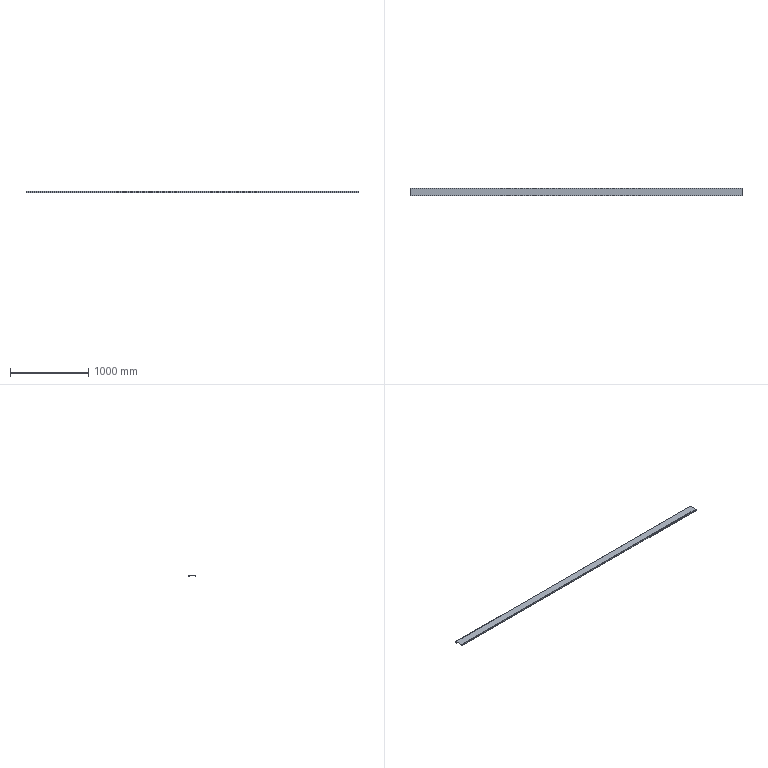Part | STEP file | E3-粉仓踢脚Plate 8 | 1 solid | 18 faces | box 4230 x 100 x 20 mm | volume 972350 mm3 | plane 12 | cylinder 6 | commonest cylinder face diameters 2 x3 5 x3
STEP:
#1=CARTESIAN_POINT('',(0.,0.,0.));
#2=DIRECTION('',(0.,0.,1.));
#3=DIRECTION('',(1.,0.,0.));
#4=AXIS2_PLACEMENT_3D('',#1,#2,#3);
#5=CARTESIAN_POINT('',(-2115.,1.5,-2.5));
#6=VERTEX_POINT('',#5);
#7=CARTESIAN_POINT('',(-2115.,1.5,-20.));
#8=VERTEX_POINT('',#7);
#9=CARTESIAN_POINT('',(-2115.,1.5,-2.5));
#10=DIRECTION('',(0.,0.,-1.));
#11=VECTOR('',#10,1.);
#12=LINE('',#9,#11);
#13=CARTESIAN_POINT('',(2115.,1.5,-2.5));
#14=DIRECTION('',(0.,-1.,0.));
#15=DIRECTION('',(0.,0.,1.));
#16=AXIS2_PLACEMENT_3D('',#13,#14,#15);
#17=PLANE('',#16);
#18=CARTESIAN_POINT('',(0.,4230.));
#19=DIRECTION('',(-1.,0.));
#20=VECTOR('',#19,1.);
#21=LINE('',#18,#20);
#22=(GEOMETRIC_REPRESENTATION_CONTEXT(2)PARAMETRIC_REPRESENTATION_CONTEXT()REPRESENTATION_CONTEXT('',''));
#23=DEFINITIONAL_REPRESENTATION('',(#21),#22);
#24=PCURVE('',#17,#23);
#25=CARTESIAN_POINT('',(-2115.,2.5,-2.5));
#26=DIRECTION('',(-1.,0.,0.));
#27=DIRECTION('',(0.,0.,-1.));
#28=AXIS2_PLACEMENT_3D('',#25,#26,#27);
#29=PLANE('',#28);
#30=CARTESIAN_POINT('',(0.,1.));
#31=DIRECTION('',(1.,0.));
#32=VECTOR('',#31,1.);
#33=LINE('',#30,#32);
#34=(GEOMETRIC_REPRESENTATION_CONTEXT(2)PARAMETRIC_REPRESENTATION_CONTEXT()REPRESENTATION_CONTEXT('',''));
#35=DEFINITIONAL_REPRESENTATION('',(#33),#34);
#36=PCURVE('',#29,#35);
#37=SURFACE_CURVE('',#12,(#24,#36),.PCURVE_S1.);
#38=EDGE_CURVE('',#6,#8,#37,.T.);
#39=ORIENTED_EDGE('',*,*,#38,.F.);
#40=CARTESIAN_POINT('',(2115.,1.5,-2.5));
#41=VERTEX_POINT('',#40);
#42=CARTESIAN_POINT('',(2115.,1.5,-2.5));
#43=DIRECTION('',(-1.,0.,0.));
#44=VECTOR('',#43,1.);
#45=LINE('',#42,#44);
#46=CARTESIAN_POINT('',(0.,0.));
#47=DIRECTION('',(0.,1.));
#48=VECTOR('',#47,1.);
#49=LINE('',#46,#48);
#50=(GEOMETRIC_REPRESENTATION_CONTEXT(2)PARAMETRIC_REPRESENTATION_CONTEXT()REPRESENTATION_CONTEXT('',''));
#51=DEFINITIONAL_REPRESENTATION('',(#49),#50);
#52=PCURVE('',#17,#51);
#53=CARTESIAN_POINT('',(2115.,2.5,-2.5));
#54=DIRECTION('',(-1.,0.,0.));
#55=DIRECTION('',(0.,0.,-1.));
#56=AXIS2_PLACEMENT_3D('',#53,#54,#55);
#57=CYLINDRICAL_SURFACE('',#56,1.);
#58=CARTESIAN_POINT('',(1.571,0.));
#59=DIRECTION('',(0.,1.));
#60=VECTOR('',#59,1.);
#61=LINE('',#58,#60);
#62=(GEOMETRIC_REPRESENTATION_CONTEXT(2)PARAMETRIC_REPRESENTATION_CONTEXT()REPRESENTATION_CONTEXT('',''));
#63=DEFINITIONAL_REPRESENTATION('',(#61),#62);
#64=PCURVE('',#57,#63);
#65=SURFACE_CURVE('',#45,(#52,#64),.PCURVE_S1.);
#66=EDGE_CURVE('',#41,#6,#65,.T.);
#67=ORIENTED_EDGE('',*,*,#66,.F.);
#68=CARTESIAN_POINT('',(2115.,1.5,-20.));
#69=VERTEX_POINT('',#68);
#70=CARTESIAN_POINT('',(2115.,1.5,-2.5));
#71=DIRECTION('',(0.,0.,-1.));
#72=VECTOR('',#71,1.);
#73=LINE('',#70,#72);
#74=CARTESIAN_POINT('',(0.,0.));
#75=DIRECTION('',(-1.,0.));
#76=VECTOR('',#75,1.);
#77=LINE('',#74,#76);
#78=(GEOMETRIC_REPRESENTATION_CONTEXT(2)PARAMETRIC_REPRESENTATION_CONTEXT()REPRESENTATION_CONTEXT('',''));
#79=DEFINITIONAL_REPRESENTATION('',(#77),#78);
#80=PCURVE('',#17,#79);
#81=CARTESIAN_POINT('',(2115.,2.5,-2.5));
#82=DIRECTION('',(-1.,0.,0.));
#83=DIRECTION('',(0.,0.,-1.));
#84=AXIS2_PLACEMENT_3D('',#81,#82,#83);
#85=PLANE('',#84);
#86=CARTESIAN_POINT('',(0.,1.));
#87=DIRECTION('',(1.,0.));
#88=VECTOR('',#87,1.);
#89=LINE('',#86,#88);
#90=(GEOMETRIC_REPRESENTATION_CONTEXT(2)PARAMETRIC_REPRESENTATION_CONTEXT()REPRESENTATION_CONTEXT('',''));
#91=DEFINITIONAL_REPRESENTATION('',(#89),#90);
#92=PCURVE('',#85,#91);
#93=SURFACE_CURVE('',#73,(#80,#92),.PCURVE_S1.);
#94=EDGE_CURVE('',#41,#69,#93,.T.);
#95=ORIENTED_EDGE('',*,*,#94,.T.);
#96=CARTESIAN_POINT('',(2115.,1.5,-20.));
#97=DIRECTION('',(-1.,0.,0.));
#98=VECTOR('',#97,1.);
#99=LINE('',#96,#98);
#100=CARTESIAN_POINT('',(-17.5,0.));
#101=DIRECTION('',(0.,1.));
#102=VECTOR('',#101,1.);
#103=LINE('',#100,#102);
#104=(GEOMETRIC_REPRESENTATION_CONTEXT(2)PARAMETRIC_REPRESENTATION_CONTEXT()REPRESENTATION_CONTEXT('',''));
#105=DEFINITIONAL_REPRESENTATION('',(#103),#104);
#106=PCURVE('',#17,#105);
#107=CARTESIAN_POINT('',(2115.,0.,-20.));
#108=DIRECTION('',(0.,0.,-1.));
#109=DIRECTION('',(1.,0.,0.));
#110=AXIS2_PLACEMENT_3D('',#107,#108,#109);
#111=PLANE('',#110);
#112=CARTESIAN_POINT('',(0.,-1.5));
#113=DIRECTION('',(-1.,0.));
#114=VECTOR('',#113,1.);
#115=LINE('',#112,#114);
#116=(GEOMETRIC_REPRESENTATION_CONTEXT(2)PARAMETRIC_REPRESENTATION_CONTEXT()REPRESENTATION_CONTEXT('',''));
#117=DEFINITIONAL_REPRESENTATION('',(#115),#116);
#118=PCURVE('',#111,#117);
#119=SURFACE_CURVE('',#99,(#106,#118),.PCURVE_S1.);
#120=EDGE_CURVE('',#69,#8,#119,.T.);
#121=ORIENTED_EDGE('',*,*,#120,.T.);
#122=EDGE_LOOP('',(#39,#67,#95,#121));
#123=FACE_BOUND('',#122,.T.);
#124=ADVANCED_FACE('',(#123),#17,.F.);
#125=CARTESIAN_POINT('',(-2115.,0.,-20.));
#126=VERTEX_POINT('',#125);
#127=CARTESIAN_POINT('',(-2115.,0.,-20.));
#128=DIRECTION('',(0.,1.,0.));
#129=VECTOR('',#128,1.);
#130=LINE('',#127,#129);
#131=CARTESIAN_POINT('',(-4230.,0.));
#132=DIRECTION('',(0.,-1.));
#133=VECTOR('',#132,1.);
#134=LINE('',#131,#133);
#135=(GEOMETRIC_REPRESENTATION_CONTEXT(2)PARAMETRIC_REPRESENTATION_CONTEXT()REPRESENTATION_CONTEXT('',''));
#136=DEFINITIONAL_REPRESENTATION('',(#134),#135);
#137=PCURVE('',#111,#136);
#138=CARTESIAN_POINT('',(17.5,2.5));
#139=DIRECTION('',(0.,-1.));
#140=VECTOR('',#139,1.);
#141=LINE('',#138,#140);
#142=(GEOMETRIC_REPRESENTATION_CONTEXT(2)PARAMETRIC_REPRESENTATION_CONTEXT()REPRESENTATION_CONTEXT('',''));
#143=DEFINITIONAL_REPRESENTATION('',(#141),#142);
#144=PCURVE('',#29,#143);
#145=SURFACE_CURVE('',#130,(#137,#144),.PCURVE_S1.);
#146=EDGE_CURVE('',#126,#8,#145,.T.);
#147=ORIENTED_EDGE('',*,*,#146,.T.);
#148=ORIENTED_EDGE('',*,*,#120,.F.);
#149=CARTESIAN_POINT('',(2115.,0.,-20.));
#150=VERTEX_POINT('',#149);
#151=CARTESIAN_POINT('',(2115.,0.,-20.));
#152=DIRECTION('',(0.,1.,0.));
#153=VECTOR('',#152,1.);
#154=LINE('',#151,#153);
#155=CARTESIAN_POINT('',(0.,0.));
#156=DIRECTION('',(0.,-1.));
#157=VECTOR('',#156,1.);
#158=LINE('',#155,#157);
#159=(GEOMETRIC_REPRESENTATION_CONTEXT(2)PARAMETRIC_REPRESENTATION_CONTEXT()REPRESENTATION_CONTEXT('',''));
#160=DEFINITIONAL_REPRESENTATION('',(#158),#159);
#161=PCURVE('',#111,#160);
#162=CARTESIAN_POINT('',(17.5,2.5));
#163=DIRECTION('',(0.,-1.));
#164=VECTOR('',#163,1.);
#165=LINE('',#162,#164);
#166=(GEOMETRIC_REPRESENTATION_CONTEXT(2)PARAMETRIC_REPRESENTATION_CONTEXT()REPRESENTATION_CONTEXT('',''));
#167=DEFINITIONAL_REPRESENTATION('',(#165),#166);
#168=PCURVE('',#85,#167);
#169=SURFACE_CURVE('',#154,(#161,#168),.PCURVE_S1.);
#170=EDGE_CURVE('',#150,#69,#169,.T.);
#171=ORIENTED_EDGE('',*,*,#170,.F.);
#172=CARTESIAN_POINT('',(2115.,0.,-20.));
#173=DIRECTION('',(-1.,0.,0.));
#174=VECTOR('',#173,1.);
#175=LINE('',#172,#174);
#176=CARTESIAN_POINT('',(0.,0.));
#177=DIRECTION('',(-1.,0.));
#178=VECTOR('',#177,1.);
#179=LINE('',#176,#178);
#180=(GEOMETRIC_REPRESENTATION_CONTEXT(2)PARAMETRIC_REPRESENTATION_CONTEXT()REPRESENTATION_CONTEXT('',''));
#181=DEFINITIONAL_REPRESENTATION('',(#179),#180);
#182=PCURVE('',#111,#181);
#183=CARTESIAN_POINT('',(2115.,0.,-2.5));
#184=DIRECTION('',(0.,-1.,0.));
#185=DIRECTION('',(0.,0.,1.));
#186=AXIS2_PLACEMENT_3D('',#183,#184,#185);
#187=PLANE('',#186);
#188=CARTESIAN_POINT('',(-17.5,0.));
#189=DIRECTION('',(0.,1.));
#190=VECTOR('',#189,1.);
#191=LINE('',#188,#190);
#192=(GEOMETRIC_REPRESENTATION_CONTEXT(2)PARAMETRIC_REPRESENTATION_CONTEXT()REPRESENTATION_CONTEXT('',''));
#193=DEFINITIONAL_REPRESENTATION('',(#191),#192);
#194=PCURVE('',#187,#193);
#195=SURFACE_CURVE('',#175,(#182,#194),.PCURVE_S1.);
#196=EDGE_CURVE('',#150,#126,#195,.T.);
#197=ORIENTED_EDGE('',*,*,#196,.T.);
#198=EDGE_LOOP('',(#147,#148,#171,#197));
#199=FACE_BOUND('',#198,.T.);
#200=ADVANCED_FACE('',(#199),#111,.T.);
#201=CARTESIAN_POINT('',(-2115.,0.,-2.5));
#202=VERTEX_POINT('',#201);
#203=CARTESIAN_POINT('',(-2115.,0.,-2.5));
#204=DIRECTION('',(0.,0.,-1.));
#205=VECTOR('',#204,1.);
#206=LINE('',#203,#205);
#207=CARTESIAN_POINT('',(0.,4230.));
#208=DIRECTION('',(-1.,0.));
#209=VECTOR('',#208,1.);
#210=LINE('',#207,#209);
#211=(GEOMETRIC_REPRESENTATION_CONTEXT(2)PARAMETRIC_REPRESENTATION_CONTEXT()REPRESENTATION_CONTEXT('',''));
#212=DEFINITIONAL_REPRESENTATION('',(#210),#211);
#213=PCURVE('',#187,#212);
#214=CARTESIAN_POINT('',(0.,2.5));
#215=DIRECTION('',(1.,0.));
#216=VECTOR('',#215,1.);
#217=LINE('',#214,#216);
#218=(GEOMETRIC_REPRESENTATION_CONTEXT(2)PARAMETRIC_REPRESENTATION_CONTEXT()REPRESENTATION_CONTEXT('',''));
#219=DEFINITIONAL_REPRESENTATION('',(#217),#218);
#220=PCURVE('',#29,#219);
#221=SURFACE_CURVE('',#206,(#213,#220),.PCURVE_S1.);
#222=EDGE_CURVE('',#202,#126,#221,.T.);
#223=ORIENTED_EDGE('',*,*,#222,.T.);
#224=ORIENTED_EDGE('',*,*,#196,.F.);
#225=CARTESIAN_POINT('',(2115.,0.,-2.5));
#226=VERTEX_POINT('',#225);
#227=CARTESIAN_POINT('',(2115.,0.,-2.5));
#228=DIRECTION('',(0.,0.,-1.));
#229=VECTOR('',#228,1.);
#230=LINE('',#227,#229);
#231=CARTESIAN_POINT('',(0.,0.));
#232=DIRECTION('',(-1.,0.));
#233=VECTOR('',#232,1.);
#234=LINE('',#231,#233);
#235=(GEOMETRIC_REPRESENTATION_CONTEXT(2)PARAMETRIC_REPRESENTATION_CONTEXT()REPRESENTATION_CONTEXT('',''));
#236=DEFINITIONAL_REPRESENTATION('',(#234),#235);
#237=PCURVE('',#187,#236);
#238=CARTESIAN_POINT('',(0.,2.5));
#239=DIRECTION('',(1.,0.));
#240=VECTOR('',#239,1.);
#241=LINE('',#238,#240);
#242=(GEOMETRIC_REPRESENTATION_CONTEXT(2)PARAMETRIC_REPRESENTATION_CONTEXT()REPRESENTATION_CONTEXT('',''));
#243=DEFINITIONAL_REPRESENTATION('',(#241),#242);
#244=PCURVE('',#85,#243);
#245=SURFACE_CURVE('',#230,(#237,#244),.PCURVE_S1.);
#246=EDGE_CURVE('',#226,#150,#245,.T.);
#247=ORIENTED_EDGE('',*,*,#246,.F.);
#248=CARTESIAN_POINT('',(2115.,0.,-2.5));
#249=DIRECTION('',(-1.,0.,0.));
#250=VECTOR('',#249,1.);
#251=LINE('',#248,#250);
#252=CARTESIAN_POINT('',(0.,0.));
#253=DIRECTION('',(0.,1.));
#254=VECTOR('',#253,1.);
#255=LINE('',#252,#254);
#256=(GEOMETRIC_REPRESENTATION_CONTEXT(2)PARAMETRIC_REPRESENTATION_CONTEXT()REPRESENTATION_CONTEXT('',''));
#257=DEFINITIONAL_REPRESENTATION('',(#255),#256);
#258=PCURVE('',#187,#257);
#259=CARTESIAN_POINT('',(2115.,2.5,-2.5));
#260=DIRECTION('',(-1.,0.,0.));
#261=DIRECTION('',(0.,0.,-1.));
#262=AXIS2_PLACEMENT_3D('',#259,#260,#261);
#263=CYLINDRICAL_SURFACE('',#262,2.5);
#264=CARTESIAN_POINT('',(1.571,0.));
#265=DIRECTION('',(0.,1.));
#266=VECTOR('',#265,1.);
#267=LINE('',#264,#266);
#268=(GEOMETRIC_REPRESENTATION_CONTEXT(2)PARAMETRIC_REPRESENTATION_CONTEXT()REPRESENTATION_CONTEXT('',''));
#269=DEFINITIONAL_REPRESENTATION('',(#267),#268);
#270=PCURVE('',#263,#269);
#271=SURFACE_CURVE('',#251,(#258,#270),.PCURVE_S1.);
#272=EDGE_CURVE('',#226,#202,#271,.T.);
#273=ORIENTED_EDGE('',*,*,#272,.T.);
#274=EDGE_LOOP('',(#223,#224,#247,#273));
#275=FACE_BOUND('',#274,.T.);
#276=ADVANCED_FACE('',(#275),#187,.T.);
#277=CARTESIAN_POINT('',(-2115.,2.5,0.));
#278=VERTEX_POINT('',#277);
#279=CARTESIAN_POINT('',(-2115.,2.5,-2.5));
#280=DIRECTION('',(1.,0.,0.));
#281=DIRECTION('',(0.,0.,-1.));
#282=AXIS2_PLACEMENT_3D('',#279,#280,#281);
#283=CIRCLE('',#282,2.5);
#284=CARTESIAN_POINT('',(6.283,4230.));
#285=DIRECTION('',(-1.,0.));
#286=VECTOR('',#285,1.);
#287=LINE('',#284,#286);
#288=(GEOMETRIC_REPRESENTATION_CONTEXT(2)PARAMETRIC_REPRESENTATION_CONTEXT()REPRESENTATION_CONTEXT('',''));
#289=DEFINITIONAL_REPRESENTATION('',(#287),#288);
#290=PCURVE('',#263,#289);
#291=CARTESIAN_POINT('',(2.5,0.));
#292=CARTESIAN_POINT('',(2.5,-4.33));
#293=CARTESIAN_POINT('',(-1.25,-2.165));
#294=CARTESIAN_POINT('',(-5.,0.));
#295=CARTESIAN_POINT('',(-1.25,2.165));
#296=CARTESIAN_POINT('',(2.5,4.33));
#297=CARTESIAN_POINT('',(2.5,0.));
#298=(BOUNDED_CURVE()B_SPLINE_CURVE(2,(#291,#292,#293,#294,#295,#296,#297),.UNSPECIFIED.,.T.,.F.)B_SPLINE_CURVE_WITH_KNOTS((1,2,2,2,2,1),(-2.094,0.,2.094,4.189,6.283,8.378),.UNSPECIFIED.)CURVE()GEOMETRIC_REPRESENTATION_ITEM()RATIONAL_B_SPLINE_CURVE((1.,0.5,1.,0.5,1.,0.5,1.))REPRESENTATION_ITEM(''));
#299=(GEOMETRIC_REPRESENTATION_CONTEXT(2)PARAMETRIC_REPRESENTATION_CONTEXT()REPRESENTATION_CONTEXT('',''));
#300=DEFINITIONAL_REPRESENTATION('',(#298),#299);
#301=PCURVE('',#29,#300);
#302=SURFACE_CURVE('',#283,(#290,#301),.PCURVE_S1.);
#303=EDGE_CURVE('',#278,#202,#302,.T.);
#304=ORIENTED_EDGE('',*,*,#303,.T.);
#305=ORIENTED_EDGE('',*,*,#272,.F.);
#306=CARTESIAN_POINT('',(2115.,2.5,0.));
#307=VERTEX_POINT('',#306);
#308=CARTESIAN_POINT('',(2115.,2.5,-2.5));
#309=DIRECTION('',(1.,0.,0.));
#310=DIRECTION('',(0.,0.,-1.));
#311=AXIS2_PLACEMENT_3D('',#308,#309,#310);
#312=CIRCLE('',#311,2.5);
#313=CARTESIAN_POINT('',(6.283,0.));
#314=DIRECTION('',(-1.,0.));
#315=VECTOR('',#314,1.);
#316=LINE('',#313,#315);
#317=(GEOMETRIC_REPRESENTATION_CONTEXT(2)PARAMETRIC_REPRESENTATION_CONTEXT()REPRESENTATION_CONTEXT('',''));
#318=DEFINITIONAL_REPRESENTATION('',(#316),#317);
#319=PCURVE('',#263,#318);
#320=CARTESIAN_POINT('',(2.5,0.));
#321=CARTESIAN_POINT('',(2.5,-4.33));
#322=CARTESIAN_POINT('',(-1.25,-2.165));
#323=CARTESIAN_POINT('',(-5.,0.));
#324=CARTESIAN_POINT('',(-1.25,2.165));
#325=CARTESIAN_POINT('',(2.5,4.33));
#326=CARTESIAN_POINT('',(2.5,0.));
#327=(BOUNDED_CURVE()B_SPLINE_CURVE(2,(#320,#321,#322,#323,#324,#325,#326),.UNSPECIFIED.,.T.,.F.)B_SPLINE_CURVE_WITH_KNOTS((1,2,2,2,2,1),(-2.094,0.,2.094,4.189,6.283,8.378),.UNSPECIFIED.)CURVE()GEOMETRIC_REPRESENTATION_ITEM()RATIONAL_B_SPLINE_CURVE((1.,0.5,1.,0.5,1.,0.5,1.))REPRESENTATION_ITEM(''));
#328=(GEOMETRIC_REPRESENTATION_CONTEXT(2)PARAMETRIC_REPRESENTATION_CONTEXT()REPRESENTATION_CONTEXT('',''));
#329=DEFINITIONAL_REPRESENTATION('',(#327),#328);
#330=PCURVE('',#85,#329);
#331=SURFACE_CURVE('',#312,(#319,#330),.PCURVE_S1.);
#332=EDGE_CURVE('',#307,#226,#331,.T.);
#333=ORIENTED_EDGE('',*,*,#332,.F.);
#334=CARTESIAN_POINT('',(2115.,2.5,0.));
#335=DIRECTION('',(-1.,0.,0.));
#336=VECTOR('',#335,1.);
#337=LINE('',#334,#336);
#338=CARTESIAN_POINT('',(3.142,0.));
#339=DIRECTION('',(0.,1.));
#340=VECTOR('',#339,1.);
#341=LINE('',#338,#340);
#342=(GEOMETRIC_REPRESENTATION_CONTEXT(2)PARAMETRIC_REPRESENTATION_CONTEXT()REPRESENTATION_CONTEXT('',''));
#343=DEFINITIONAL_REPRESENTATION('',(#341),#342);
#344=PCURVE('',#263,#343);
#345=CARTESIAN_POINT('',(2115.,2.5,0.));
#346=DIRECTION('',(0.,0.,1.));
#347=DIRECTION('',(-1.,0.,0.));
#348=AXIS2_PLACEMENT_3D('',#345,#346,#347);
#349=PLANE('',#348);
#350=CARTESIAN_POINT('',(0.,0.));
#351=DIRECTION('',(1.,0.));
#352=VECTOR('',#351,1.);
#353=LINE('',#350,#352);
#354=(GEOMETRIC_REPRESENTATION_CONTEXT(2)PARAMETRIC_REPRESENTATION_CONTEXT()REPRESENTATION_CONTEXT('',''));
#355=DEFINITIONAL_REPRESENTATION('',(#353),#354);
#356=PCURVE('',#349,#355);
#357=SURFACE_CURVE('',#337,(#344,#356),.PCURVE_S1.);
#358=EDGE_CURVE('',#307,#278,#357,.T.);
#359=ORIENTED_EDGE('',*,*,#358,.T.);
#360=EDGE_LOOP('',(#304,#305,#333,#359));
#361=FACE_BOUND('',#360,.T.);
#362=ADVANCED_FACE('',(#361),#263,.T.);
#363=CARTESIAN_POINT('',(-2115.,97.5,0.));
#364=VERTEX_POINT('',#363);
#365=CARTESIAN_POINT('',(-2115.,2.5,0.));
#366=DIRECTION('',(0.,-1.,0.));
#367=VECTOR('',#366,1.);
#368=LINE('',#365,#367);
#369=CARTESIAN_POINT('',(4230.,0.));
#370=DIRECTION('',(0.,1.));
#371=VECTOR('',#370,1.);
#372=LINE('',#369,#371);
#373=(GEOMETRIC_REPRESENTATION_CONTEXT(2)PARAMETRIC_REPRESENTATION_CONTEXT()REPRESENTATION_CONTEXT('',''));
#374=DEFINITIONAL_REPRESENTATION('',(#372),#373);
#375=PCURVE('',#349,#374);
#376=CARTESIAN_POINT('',(-2.5,0.));
#377=DIRECTION('',(0.,1.));
#378=VECTOR('',#377,1.);
#379=LINE('',#376,#378);
#380=(GEOMETRIC_REPRESENTATION_CONTEXT(2)PARAMETRIC_REPRESENTATION_CONTEXT()REPRESENTATION_CONTEXT('',''));
#381=DEFINITIONAL_REPRESENTATION('',(#379),#380);
#382=PCURVE('',#29,#381);
#383=SURFACE_CURVE('',#368,(#375,#382),.PCURVE_S1.);
#384=EDGE_CURVE('',#364,#278,#383,.T.);
#385=ORIENTED_EDGE('',*,*,#384,.T.);
#386=ORIENTED_EDGE('',*,*,#358,.F.);
#387=CARTESIAN_POINT('',(2115.,97.5,0.));
#388=VERTEX_POINT('',#387);
#389=CARTESIAN_POINT('',(2115.,2.5,0.));
#390=DIRECTION('',(0.,-1.,0.));
#391=VECTOR('',#390,1.);
#392=LINE('',#389,#391);
#393=CARTESIAN_POINT('',(0.,0.));
#394=DIRECTION('',(0.,1.));
#395=VECTOR('',#394,1.);
#396=LINE('',#393,#395);
#397=(GEOMETRIC_REPRESENTATION_CONTEXT(2)PARAMETRIC_REPRESENTATION_CONTEXT()REPRESENTATION_CONTEXT('',''));
#398=DEFINITIONAL_REPRESENTATION('',(#396),#397);
#399=PCURVE('',#349,#398);
#400=CARTESIAN_POINT('',(-2.5,0.));
#401=DIRECTION('',(0.,1.));
#402=VECTOR('',#401,1.);
#403=LINE('',#400,#402);
#404=(GEOMETRIC_REPRESENTATION_CONTEXT(2)PARAMETRIC_REPRESENTATION_CONTEXT()REPRESENTATION_CONTEXT('',''));
#405=DEFINITIONAL_REPRESENTATION('',(#403),#404);
#406=PCURVE('',#85,#405);
#407=SURFACE_CURVE('',#392,(#399,#406),.PCURVE_S1.);
#408=EDGE_CURVE('',#388,#307,#407,.T.);
#409=ORIENTED_EDGE('',*,*,#408,.F.);
#410=CARTESIAN_POINT('',(2115.,97.5,0.));
#411=DIRECTION('',(-1.,0.,0.));
#412=VECTOR('',#411,1.);
#413=LINE('',#410,#412);
#414=CARTESIAN_POINT('',(0.,-95.));
#415=DIRECTION('',(1.,0.));
#416=VECTOR('',#415,1.);
#417=LINE('',#414,#416);
#418=(GEOMETRIC_REPRESENTATION_CONTEXT(2)PARAMETRIC_REPRESENTATION_CONTEXT()REPRESENTATION_CONTEXT('',''));
#419=DEFINITIONAL_REPRESENTATION('',(#417),#418);
#420=PCURVE('',#349,#419);
#421=CARTESIAN_POINT('',(2115.,97.5,-2.5));
#422=DIRECTION('',(-1.,0.,0.));
#423=DIRECTION('',(0.,0.,-1.));
#424=AXIS2_PLACEMENT_3D('',#421,#422,#423);
#425=CYLINDRICAL_SURFACE('',#424,2.5);
#426=CARTESIAN_POINT('',(3.142,0.));
#427=DIRECTION('',(0.,1.));
#428=VECTOR('',#427,1.);
#429=LINE('',#426,#428);
#430=(GEOMETRIC_REPRESENTATION_CONTEXT(2)PARAMETRIC_REPRESENTATION_CONTEXT()REPRESENTATION_CONTEXT('',''));
#431=DEFINITIONAL_REPRESENTATION('',(#429),#430);
#432=PCURVE('',#425,#431);
#433=SURFACE_CURVE('',#413,(#420,#432),.PCURVE_S1.);
#434=EDGE_CURVE('',#388,#364,#433,.T.);
#435=ORIENTED_EDGE('',*,*,#434,.T.);
#436=EDGE_LOOP('',(#385,#386,#409,#435));
#437=FACE_BOUND('',#436,.T.);
#438=ADVANCED_FACE('',(#437),#349,.T.);
#439=CARTESIAN_POINT('',(-2115.,100.,-2.5));
#440=VERTEX_POINT('',#439);
#441=CARTESIAN_POINT('',(-2115.,97.5,-2.5));
#442=DIRECTION('',(1.,0.,0.));
#443=DIRECTION('',(0.,0.,1.));
#444=AXIS2_PLACEMENT_3D('',#441,#442,#443);
#445=CIRCLE('',#444,2.5);
#446=CARTESIAN_POINT('',(9.425,4230.));
#447=DIRECTION('',(-1.,0.));
#448=VECTOR('',#447,1.);
#449=LINE('',#446,#448);
#450=(GEOMETRIC_REPRESENTATION_CONTEXT(2)PARAMETRIC_REPRESENTATION_CONTEXT()REPRESENTATION_CONTEXT('',''));
#451=DEFINITIONAL_REPRESENTATION('',(#449),#450);
#452=PCURVE('',#425,#451);
#453=CARTESIAN_POINT('',(-2.5,-95.));
#454=CARTESIAN_POINT('',(-2.5,-90.67));
#455=CARTESIAN_POINT('',(1.25,-92.835));
#456=CARTESIAN_POINT('',(5.,-95.));
#457=CARTESIAN_POINT('',(1.25,-97.165));
#458=CARTESIAN_POINT('',(-2.5,-99.33));
#459=CARTESIAN_POINT('',(-2.5,-95.));
#460=(BOUNDED_CURVE()B_SPLINE_CURVE(2,(#453,#454,#455,#456,#457,#458,#459),.UNSPECIFIED.,.T.,.F.)B_SPLINE_CURVE_WITH_KNOTS((1,2,2,2,2,1),(-2.094,0.,2.094,4.189,6.283,8.378),.UNSPECIFIED.)CURVE()GEOMETRIC_REPRESENTATION_ITEM()RATIONAL_B_SPLINE_CURVE((1.,0.5,1.,0.5,1.,0.5,1.))REPRESENTATION_ITEM(''));
#461=(GEOMETRIC_REPRESENTATION_CONTEXT(2)PARAMETRIC_REPRESENTATION_CONTEXT()REPRESENTATION_CONTEXT('',''));
#462=DEFINITIONAL_REPRESENTATION('',(#460),#461);
#463=PCURVE('',#29,#462);
#464=SURFACE_CURVE('',#445,(#452,#463),.PCURVE_S1.);
#465=EDGE_CURVE('',#440,#364,#464,.T.);
#466=ORIENTED_EDGE('',*,*,#465,.T.);
#467=ORIENTED_EDGE('',*,*,#434,.F.);
#468=CARTESIAN_POINT('',(2115.,100.,-2.5));
#469=VERTEX_POINT('',#468);
#470=CARTESIAN_POINT('',(2115.,97.5,-2.5));
#471=DIRECTION('',(1.,0.,0.));
#472=DIRECTION('',(0.,0.,1.));
#473=AXIS2_PLACEMENT_3D('',#470,#471,#472);
#474=CIRCLE('',#473,2.5);
#475=CARTESIAN_POINT('',(9.425,0.));
#476=DIRECTION('',(-1.,0.));
#477=VECTOR('',#476,1.);
#478=LINE('',#475,#477);
#479=(GEOMETRIC_REPRESENTATION_CONTEXT(2)PARAMETRIC_REPRESENTATION_CONTEXT()REPRESENTATION_CONTEXT('',''));
#480=DEFINITIONAL_REPRESENTATION('',(#478),#479);
#481=PCURVE('',#425,#480);
#482=CARTESIAN_POINT('',(-2.5,-95.));
#483=CARTESIAN_POINT('',(-2.5,-90.67));
#484=CARTESIAN_POINT('',(1.25,-92.835));
#485=CARTESIAN_POINT('',(5.,-95.));
#486=CARTESIAN_POINT('',(1.25,-97.165));
#487=CARTESIAN_POINT('',(-2.5,-99.33));
#488=CARTESIAN_POINT('',(-2.5,-95.));
#489=(BOUNDED_CURVE()B_SPLINE_CURVE(2,(#482,#483,#484,#485,#486,#487,#488),.UNSPECIFIED.,.T.,.F.)B_SPLINE_CURVE_WITH_KNOTS((1,2,2,2,2,1),(-2.094,0.,2.094,4.189,6.283,8.378),.UNSPECIFIED.)CURVE()GEOMETRIC_REPRESENTATION_ITEM()RATIONAL_B_SPLINE_CURVE((1.,0.5,1.,0.5,1.,0.5,1.))REPRESENTATION_ITEM(''));
#490=(GEOMETRIC_REPRESENTATION_CONTEXT(2)PARAMETRIC_REPRESENTATION_CONTEXT()REPRESENTATION_CONTEXT('',''));
#491=DEFINITIONAL_REPRESENTATION('',(#489),#490);
#492=PCURVE('',#85,#491);
#493=SURFACE_CURVE('',#474,(#481,#492),.PCURVE_S1.);
#494=EDGE_CURVE('',#469,#388,#493,.T.);
#495=ORIENTED_EDGE('',*,*,#494,.F.);
#496=CARTESIAN_POINT('',(2115.,100.,-2.5));
#497=DIRECTION('',(-1.,0.,0.));
#498=VECTOR('',#497,1.);
#499=LINE('',#496,#498);
#500=CARTESIAN_POINT('',(4.712,0.));
#501=DIRECTION('',(0.,1.));
#502=VECTOR('',#501,1.);
#503=LINE('',#500,#502);
#504=(GEOMETRIC_REPRESENTATION_CONTEXT(2)PARAMETRIC_REPRESENTATION_CONTEXT()REPRESENTATION_CONTEXT('',''));
#505=DEFINITIONAL_REPRESENTATION('',(#503),#504);
#506=PCURVE('',#425,#505);
#507=CARTESIAN_POINT('',(2115.,100.,-2.5));
#508=DIRECTION('',(0.,1.,0.));
#509=DIRECTION('',(0.,0.,-1.));
#510=AXIS2_PLACEMENT_3D('',#507,#508,#509);
#511=PLANE('',#510);
#512=CARTESIAN_POINT('',(0.,0.));
#513=DIRECTION('',(0.,1.));
#514=VECTOR('',#513,1.);
#515=LINE('',#512,#514);
#516=(GEOMETRIC_REPRESENTATION_CONTEXT(2)PARAMETRIC_REPRESENTATION_CONTEXT()REPRESENTATION_CONTEXT('',''));
#517=DEFINITIONAL_REPRESENTATION('',(#515),#516);
#518=PCURVE('',#511,#517);
#519=SURFACE_CURVE('',#499,(#506,#518),.PCURVE_S1.);
#520=EDGE_CURVE('',#469,#440,#519,.T.);
#521=ORIENTED_EDGE('',*,*,#520,.T.);
#522=EDGE_LOOP('',(#466,#467,#495,#521));
#523=FACE_BOUND('',#522,.T.);
#524=ADVANCED_FACE('',(#523),#425,.T.);
#525=CARTESIAN_POINT('',(-2115.,100.,-17.5));
#526=VERTEX_POINT('',#525);
#527=CARTESIAN_POINT('',(-2115.,100.,-2.5));
#528=DIRECTION('',(0.,0.,1.));
#529=VECTOR('',#528,1.);
#530=LINE('',#527,#529);
#531=CARTESIAN_POINT('',(0.,4230.));
#532=DIRECTION('',(-1.,0.));
#533=VECTOR('',#532,1.);
#534=LINE('',#531,#533);
#535=(GEOMETRIC_REPRESENTATION_CONTEXT(2)PARAMETRIC_REPRESENTATION_CONTEXT()REPRESENTATION_CONTEXT('',''));
#536=DEFINITIONAL_REPRESENTATION('',(#534),#535);
#537=PCURVE('',#511,#536);
#538=CARTESIAN_POINT('',(0.,-97.5));
#539=DIRECTION('',(-1.,0.));
#540=VECTOR('',#539,1.);
#541=LINE('',#538,#540);
#542=(GEOMETRIC_REPRESENTATION_CONTEXT(2)PARAMETRIC_REPRESENTATION_CONTEXT()REPRESENTATION_CONTEXT('',''));
#543=DEFINITIONAL_REPRESENTATION('',(#541),#542);
#544=PCURVE('',#29,#543);
#545=SURFACE_CURVE('',#530,(#537,#544),.PCURVE_S1.);
#546=EDGE_CURVE('',#526,#440,#545,.T.);
#547=ORIENTED_EDGE('',*,*,#546,.T.);
#548=ORIENTED_EDGE('',*,*,#520,.F.);
#549=CARTESIAN_POINT('',(2115.,100.,-17.5));
#550=VERTEX_POINT('',#549);
#551=CARTESIAN_POINT('',(2115.,100.,-2.5));
#552=DIRECTION('',(0.,0.,1.));
#553=VECTOR('',#552,1.);
#554=LINE('',#551,#553);
#555=CARTESIAN_POINT('',(0.,0.));
#556=DIRECTION('',(-1.,0.));
#557=VECTOR('',#556,1.);
#558=LINE('',#555,#557);
#559=(GEOMETRIC_REPRESENTATION_CONTEXT(2)PARAMETRIC_REPRESENTATION_CONTEXT()REPRESENTATION_CONTEXT('',''));
#560=DEFINITIONAL_REPRESENTATION('',(#558),#559);
#561=PCURVE('',#511,#560);
#562=CARTESIAN_POINT('',(0.,-97.5));
#563=DIRECTION('',(-1.,0.));
#564=VECTOR('',#563,1.);
#565=LINE('',#562,#564);
#566=(GEOMETRIC_REPRESENTATION_CONTEXT(2)PARAMETRIC_REPRESENTATION_CONTEXT()REPRESENTATION_CONTEXT('',''));
#567=DEFINITIONAL_REPRESENTATION('',(#565),#566);
#568=PCURVE('',#85,#567);
#569=SURFACE_CURVE('',#554,(#561,#568),.PCURVE_S1.);
#570=EDGE_CURVE('',#550,#469,#569,.T.);
#571=ORIENTED_EDGE('',*,*,#570,.F.);
#572=CARTESIAN_POINT('',(2115.,100.,-17.5));
#573=DIRECTION('',(-1.,0.,0.));
#574=VECTOR('',#573,1.);
#575=LINE('',#572,#574);
#576=CARTESIAN_POINT('',(15.,0.));
#577=DIRECTION('',(0.,1.));
#578=VECTOR('',#577,1.);
#579=LINE('',#576,#578);
#580=(GEOMETRIC_REPRESENTATION_CONTEXT(2)PARAMETRIC_REPRESENTATION_CONTEXT()REPRESENTATION_CONTEXT('',''));
#581=DEFINITIONAL_REPRESENTATION('',(#579),#580);
#582=PCURVE('',#511,#581);
#583=CARTESIAN_POINT('',(2115.,97.5,-17.5));
#584=DIRECTION('',(-1.,0.,0.));
#585=DIRECTION('',(0.,0.,-1.));
#586=AXIS2_PLACEMENT_3D('',#583,#584,#585);
#587=CYLINDRICAL_SURFACE('',#586,2.5);
#588=CARTESIAN_POINT('',(4.712,0.));
#589=DIRECTION('',(0.,1.));
#590=VECTOR('',#589,1.);
#591=LINE('',#588,#590);
#592=(GEOMETRIC_REPRESENTATION_CONTEXT(2)PARAMETRIC_REPRESENTATION_CONTEXT()REPRESENTATION_CONTEXT('',''));
#593=DEFINITIONAL_REPRESENTATION('',(#591),#592);
#594=PCURVE('',#587,#593);
#595=SURFACE_CURVE('',#575,(#582,#594),.PCURVE_S1.);
#596=EDGE_CURVE('',#550,#526,#595,.T.);
#597=ORIENTED_EDGE('',*,*,#596,.T.);
#598=EDGE_LOOP('',(#547,#548,#571,#597));
#599=FACE_BOUND('',#598,.T.);
#600=ADVANCED_FACE('',(#599),#511,.T.);
#601=CARTESIAN_POINT('',(-2115.,97.5,-20.));
#602=VERTEX_POINT('',#601);
#603=CARTESIAN_POINT('',(-2115.,97.5,-17.5));
#604=DIRECTION('',(1.,0.,0.));
#605=DIRECTION('',(0.,0.,1.));
#606=AXIS2_PLACEMENT_3D('',#603,#604,#605);
#607=CIRCLE('',#606,2.5);
#608=CARTESIAN_POINT('',(9.425,4230.));
#609=DIRECTION('',(-1.,0.));
#610=VECTOR('',#609,1.);
#611=LINE('',#608,#610);
#612=(GEOMETRIC_REPRESENTATION_CONTEXT(2)PARAMETRIC_REPRESENTATION_CONTEXT()REPRESENTATION_CONTEXT('',''));
#613=DEFINITIONAL_REPRESENTATION('',(#611),#612);
#614=PCURVE('',#587,#613);
#615=CARTESIAN_POINT('',(12.5,-95.));
#616=CARTESIAN_POINT('',(12.5,-90.67));
#617=CARTESIAN_POINT('',(16.25,-92.835));
#618=CARTESIAN_POINT('',(20.,-95.));
#619=CARTESIAN_POINT('',(16.25,-97.165));
#620=CARTESIAN_POINT('',(12.5,-99.33));
#621=CARTESIAN_POINT('',(12.5,-95.));
#622=(BOUNDED_CURVE()B_SPLINE_CURVE(2,(#615,#616,#617,#618,#619,#620,#621),.UNSPECIFIED.,.T.,.F.)B_SPLINE_CURVE_WITH_KNOTS((1,2,2,2,2,1),(-2.094,0.,2.094,4.189,6.283,8.378),.UNSPECIFIED.)CURVE()GEOMETRIC_REPRESENTATION_ITEM()RATIONAL_B_SPLINE_CURVE((1.,0.5,1.,0.5,1.,0.5,1.))REPRESENTATION_ITEM(''));
#623=(GEOMETRIC_REPRESENTATION_CONTEXT(2)PARAMETRIC_REPRESENTATION_CONTEXT()REPRESENTATION_CONTEXT('',''));
#624=DEFINITIONAL_REPRESENTATION('',(#622),#623);
#625=PCURVE('',#29,#624);
#626=SURFACE_CURVE('',#607,(#614,#625),.PCURVE_S1.);
#627=EDGE_CURVE('',#602,#526,#626,.T.);
#628=ORIENTED_EDGE('',*,*,#627,.T.);
#629=ORIENTED_EDGE('',*,*,#596,.F.);
#630=CARTESIAN_POINT('',(2115.,97.5,-20.));
#631=VERTEX_POINT('',#630);
#632=CARTESIAN_POINT('',(2115.,97.5,-17.5));
#633=DIRECTION('',(1.,0.,0.));
#634=DIRECTION('',(0.,0.,1.));
#635=AXIS2_PLACEMENT_3D('',#632,#633,#634);
#636=CIRCLE('',#635,2.5);
#637=CARTESIAN_POINT('',(9.425,0.));
#638=DIRECTION('',(-1.,0.));
#639=VECTOR('',#638,1.);
#640=LINE('',#637,#639);
#641=(GEOMETRIC_REPRESENTATION_CONTEXT(2)PARAMETRIC_REPRESENTATION_CONTEXT()REPRESENTATION_CONTEXT('',''));
#642=DEFINITIONAL_REPRESENTATION('',(#640),#641);
#643=PCURVE('',#587,#642);
#644=CARTESIAN_POINT('',(12.5,-95.));
#645=CARTESIAN_POINT('',(12.5,-90.67));
#646=CARTESIAN_POINT('',(16.25,-92.835));
#647=CARTESIAN_POINT('',(20.,-95.));
#648=CARTESIAN_POINT('',(16.25,-97.165));
#649=CARTESIAN_POINT('',(12.5,-99.33));
#650=CARTESIAN_POINT('',(12.5,-95.));
#651=(BOUNDED_CURVE()B_SPLINE_CURVE(2,(#644,#645,#646,#647,#648,#649,#650),.UNSPECIFIED.,.T.,.F.)B_SPLINE_CURVE_WITH_KNOTS((1,2,2,2,2,1),(-2.094,0.,2.094,4.189,6.283,8.378),.UNSPECIFIED.)CURVE()GEOMETRIC_REPRESENTATION_ITEM()RATIONAL_B_SPLINE_CURVE((1.,0.5,1.,0.5,1.,0.5,1.))REPRESENTATION_ITEM(''));
#652=(GEOMETRIC_REPRESENTATION_CONTEXT(2)PARAMETRIC_REPRESENTATION_CONTEXT()REPRESENTATION_CONTEXT('',''));
#653=DEFINITIONAL_REPRESENTATION('',(#651),#652);
#654=PCURVE('',#85,#653);
#655=SURFACE_CURVE('',#636,(#643,#654),.PCURVE_S1.);
#656=EDGE_CURVE('',#631,#550,#655,.T.);
#657=ORIENTED_EDGE('',*,*,#656,.F.);
#658=CARTESIAN_POINT('',(2115.,97.5,-20.));
#659=DIRECTION('',(-1.,0.,0.));
#660=VECTOR('',#659,1.);
#661=LINE('',#658,#660);
#662=CARTESIAN_POINT('',(6.283,0.));
#663=DIRECTION('',(0.,1.));
#664=VECTOR('',#663,1.);
#665=LINE('',#662,#664);
#666=(GEOMETRIC_REPRESENTATION_CONTEXT(2)PARAMETRIC_REPRESENTATION_CONTEXT()REPRESENTATION_CONTEXT('',''));
#667=DEFINITIONAL_REPRESENTATION('',(#665),#666);
#668=PCURVE('',#587,#667);
#669=CARTESIAN_POINT('',(2115.,97.5,-20.));
#670=DIRECTION('',(0.,0.,-1.));
#671=DIRECTION('',(1.,0.,0.));
#672=AXIS2_PLACEMENT_3D('',#669,#670,#671);
#673=PLANE('',#672);
#674=CARTESIAN_POINT('',(0.,0.));
#675=DIRECTION('',(-1.,0.));
#676=VECTOR('',#675,1.);
#677=LINE('',#674,#676);
#678=(GEOMETRIC_REPRESENTATION_CONTEXT(2)PARAMETRIC_REPRESENTATION_CONTEXT()REPRESENTATION_CONTEXT('',''));
#679=DEFINITIONAL_REPRESENTATION('',(#677),#678);
#680=PCURVE('',#673,#679);
#681=SURFACE_CURVE('',#661,(#668,#680),.PCURVE_S1.);
#682=EDGE_CURVE('',#631,#602,#681,.T.);
#683=ORIENTED_EDGE('',*,*,#682,.T.);
#684=EDGE_LOOP('',(#628,#629,#657,#683));
#685=FACE_BOUND('',#684,.T.);
#686=ADVANCED_FACE('',(#685),#587,.T.);
#687=CARTESIAN_POINT('',(-2115.,80.,-20.));
#688=VERTEX_POINT('',#687);
#689=CARTESIAN_POINT('',(-2115.,97.5,-20.));
#690=DIRECTION('',(0.,1.,0.));
#691=VECTOR('',#690,1.);
#692=LINE('',#689,#691);
#693=CARTESIAN_POINT('',(-4230.,0.));
#694=DIRECTION('',(0.,-1.));
#695=VECTOR('',#694,1.);
#696=LINE('',#693,#695);
#697=(GEOMETRIC_REPRESENTATION_CONTEXT(2)PARAMETRIC_REPRESENTATION_CONTEXT()REPRESENTATION_CONTEXT('',''));
#698=DEFINITIONAL_REPRESENTATION('',(#696),#697);
#699=PCURVE('',#673,#698);
#700=CARTESIAN_POINT('',(17.5,-95.));
#701=DIRECTION('',(0.,-1.));
#702=VECTOR('',#701,1.);
#703=LINE('',#700,#702);
#704=(GEOMETRIC_REPRESENTATION_CONTEXT(2)PARAMETRIC_REPRESENTATION_CONTEXT()REPRESENTATION_CONTEXT('',''));
#705=DEFINITIONAL_REPRESENTATION('',(#703),#704);
#706=PCURVE('',#29,#705);
#707=SURFACE_CURVE('',#692,(#699,#706),.PCURVE_S1.);
#708=EDGE_CURVE('',#688,#602,#707,.T.);
#709=ORIENTED_EDGE('',*,*,#708,.T.);
#710=ORIENTED_EDGE('',*,*,#682,.F.);
#711=CARTESIAN_POINT('',(2115.,80.,-20.));
#712=VERTEX_POINT('',#711);
#713=CARTESIAN_POINT('',(2115.,97.5,-20.));
#714=DIRECTION('',(0.,1.,0.));
#715=VECTOR('',#714,1.);
#716=LINE('',#713,#715);
#717=CARTESIAN_POINT('',(0.,0.));
#718=DIRECTION('',(0.,-1.));
#719=VECTOR('',#718,1.);
#720=LINE('',#717,#719);
#721=(GEOMETRIC_REPRESENTATION_CONTEXT(2)PARAMETRIC_REPRESENTATION_CONTEXT()REPRESENTATION_CONTEXT('',''));
#722=DEFINITIONAL_REPRESENTATION('',(#720),#721);
#723=PCURVE('',#673,#722);
#724=CARTESIAN_POINT('',(17.5,-95.));
#725=DIRECTION('',(0.,-1.));
#726=VECTOR('',#725,1.);
#727=LINE('',#724,#726);
#728=(GEOMETRIC_REPRESENTATION_CONTEXT(2)PARAMETRIC_REPRESENTATION_CONTEXT()REPRESENTATION_CONTEXT('',''));
#729=DEFINITIONAL_REPRESENTATION('',(#727),#728);
#730=PCURVE('',#85,#729);
#731=SURFACE_CURVE('',#716,(#723,#730),.PCURVE_S1.);
#732=EDGE_CURVE('',#712,#631,#731,.T.);
#733=ORIENTED_EDGE('',*,*,#732,.F.);
#734=CARTESIAN_POINT('',(2115.,80.,-20.));
#735=DIRECTION('',(-1.,0.,0.));
#736=VECTOR('',#735,1.);
#737=LINE('',#734,#736);
#738=CARTESIAN_POINT('',(0.,17.5));
#739=DIRECTION('',(-1.,0.));
#740=VECTOR('',#739,1.);
#741=LINE('',#738,#740);
#742=(GEOMETRIC_REPRESENTATION_CONTEXT(2)PARAMETRIC_REPRESENTATION_CONTEXT()REPRESENTATION_CONTEXT('',''));
#743=DEFINITIONAL_REPRESENTATION('',(#741),#742);
#744=PCURVE('',#673,#743);
#745=CARTESIAN_POINT('',(2115.,80.,-18.5));
#746=DIRECTION('',(0.,-1.,0.));
#747=DIRECTION('',(0.,0.,1.));
#748=AXIS2_PLACEMENT_3D('',#745,#746,#747);
#749=PLANE('',#748);
#750=CARTESIAN_POINT('',(-1.5,0.));
#751=DIRECTION('',(0.,1.));
#752=VECTOR('',#751,1.);
#753=LINE('',#750,#752);
#754=(GEOMETRIC_REPRESENTATION_CONTEXT(2)PARAMETRIC_REPRESENTATION_CONTEXT()REPRESENTATION_CONTEXT('',''));
#755=DEFINITIONAL_REPRESENTATION('',(#753),#754);
#756=PCURVE('',#749,#755);
#757=SURFACE_CURVE('',#737,(#744,#756),.PCURVE_S1.);
#758=EDGE_CURVE('',#712,#688,#757,.T.);
#759=ORIENTED_EDGE('',*,*,#758,.T.);
#760=EDGE_LOOP('',(#709,#710,#733,#759));
#761=FACE_BOUND('',#760,.T.);
#762=ADVANCED_FACE('',(#761),#673,.T.);
#763=CARTESIAN_POINT('',(-2115.,80.,-18.5));
#764=VERTEX_POINT('',#763);
#765=CARTESIAN_POINT('',(-2115.,80.,-18.5));
#766=DIRECTION('',(0.,0.,-1.));
#767=VECTOR('',#766,1.);
#768=LINE('',#765,#767);
#769=CARTESIAN_POINT('',(0.,4230.));
#770=DIRECTION('',(-1.,0.));
#771=VECTOR('',#770,1.);
#772=LINE('',#769,#771);
#773=(GEOMETRIC_REPRESENTATION_CONTEXT(2)PARAMETRIC_REPRESENTATION_CONTEXT()REPRESENTATION_CONTEXT('',''));
#774=DEFINITIONAL_REPRESENTATION('',(#772),#773);
#775=PCURVE('',#749,#774);
#776=CARTESIAN_POINT('',(16.,-77.5));
#777=DIRECTION('',(1.,0.));
#778=VECTOR('',#777,1.);
#779=LINE('',#776,#778);
#780=(GEOMETRIC_REPRESENTATION_CONTEXT(2)PARAMETRIC_REPRESENTATION_CONTEXT()REPRESENTATION_CONTEXT('',''));
#781=DEFINITIONAL_REPRESENTATION('',(#779),#780);
#782=PCURVE('',#29,#781);
#783=SURFACE_CURVE('',#768,(#775,#782),.PCURVE_S1.);
#784=EDGE_CURVE('',#764,#688,#783,.T.);
#785=ORIENTED_EDGE('',*,*,#784,.T.);
#786=ORIENTED_EDGE('',*,*,#758,.F.);
#787=CARTESIAN_POINT('',(2115.,80.,-18.5));
#788=VERTEX_POINT('',#787);
#789=CARTESIAN_POINT('',(2115.,80.,-18.5));
#790=DIRECTION('',(0.,0.,-1.));
#791=VECTOR('',#790,1.);
#792=LINE('',#789,#791);
#793=CARTESIAN_POINT('',(0.,0.));
#794=DIRECTION('',(-1.,0.));
#795=VECTOR('',#794,1.);
#796=LINE('',#793,#795);
#797=(GEOMETRIC_REPRESENTATION_CONTEXT(2)PARAMETRIC_REPRESENTATION_CONTEXT()REPRESENTATION_CONTEXT('',''));
#798=DEFINITIONAL_REPRESENTATION('',(#796),#797);
#799=PCURVE('',#749,#798);
#800=CARTESIAN_POINT('',(16.,-77.5));
#801=DIRECTION('',(1.,0.));
#802=VECTOR('',#801,1.);
#803=LINE('',#800,#802);
#804=(GEOMETRIC_REPRESENTATION_CONTEXT(2)PARAMETRIC_REPRESENTATION_CONTEXT()REPRESENTATION_CONTEXT('',''));
#805=DEFINITIONAL_REPRESENTATION('',(#803),#804);
#806=PCURVE('',#85,#805);
#807=SURFACE_CURVE('',#792,(#799,#806),.PCURVE_S1.);
#808=EDGE_CURVE('',#788,#712,#807,.T.);
#809=ORIENTED_EDGE('',*,*,#808,.F.);
#810=CARTESIAN_POINT('',(2115.,80.,-18.5));
#811=DIRECTION('',(-1.,0.,0.));
#812=VECTOR('',#811,1.);
#813=LINE('',#810,#812);
#814=CARTESIAN_POINT('',(0.,0.));
#815=DIRECTION('',(0.,1.));
#816=VECTOR('',#815,1.);
#817=LINE('',#814,#816);
#818=(GEOMETRIC_REPRESENTATION_CONTEXT(2)PARAMETRIC_REPRESENTATION_CONTEXT()REPRESENTATION_CONTEXT('',''));
#819=DEFINITIONAL_REPRESENTATION('',(#817),#818);
#820=PCURVE('',#749,#819);
#821=CARTESIAN_POINT('',(2115.,97.5,-18.5));
#822=DIRECTION('',(0.,0.,-1.));
#823=DIRECTION('',(1.,0.,0.));
#824=AXIS2_PLACEMENT_3D('',#821,#822,#823);
#825=PLANE('',#824);
#826=CARTESIAN_POINT('',(0.,17.5));
#827=DIRECTION('',(-1.,0.));
#828=VECTOR('',#827,1.);
#829=LINE('',#826,#828);
#830=(GEOMETRIC_REPRESENTATION_CONTEXT(2)PARAMETRIC_REPRESENTATION_CONTEXT()REPRESENTATION_CONTEXT('',''));
#831=DEFINITIONAL_REPRESENTATION('',(#829),#830);
#832=PCURVE('',#825,#831);
#833=SURFACE_CURVE('',#813,(#820,#832),.PCURVE_S1.);
#834=EDGE_CURVE('',#788,#764,#833,.T.);
#835=ORIENTED_EDGE('',*,*,#834,.T.);
#836=EDGE_LOOP('',(#785,#786,#809,#835));
#837=FACE_BOUND('',#836,.T.);
#838=ADVANCED_FACE('',(#837),#749,.T.);
#839=CARTESIAN_POINT('',(-2115.,97.5,-18.5));
#840=VERTEX_POINT('',#839);
#841=CARTESIAN_POINT('',(-2115.,97.5,-18.5));
#842=DIRECTION('',(0.,1.,0.));
#843=VECTOR('',#842,1.);
#844=LINE('',#841,#843);
#845=CARTESIAN_POINT('',(-4230.,0.));
#846=DIRECTION('',(0.,-1.));
#847=VECTOR('',#846,1.);
#848=LINE('',#845,#847);
#849=(GEOMETRIC_REPRESENTATION_CONTEXT(2)PARAMETRIC_REPRESENTATION_CONTEXT()REPRESENTATION_CONTEXT('',''));
#850=DEFINITIONAL_REPRESENTATION('',(#848),#849);
#851=PCURVE('',#825,#850);
#852=CARTESIAN_POINT('',(16.,-95.));
#853=DIRECTION('',(0.,-1.));
#854=VECTOR('',#853,1.);
#855=LINE('',#852,#854);
#856=(GEOMETRIC_REPRESENTATION_CONTEXT(2)PARAMETRIC_REPRESENTATION_CONTEXT()REPRESENTATION_CONTEXT('',''));
#857=DEFINITIONAL_REPRESENTATION('',(#855),#856);
#858=PCURVE('',#29,#857);
#859=SURFACE_CURVE('',#844,(#851,#858),.PCURVE_S1.);
#860=EDGE_CURVE('',#764,#840,#859,.T.);
#861=ORIENTED_EDGE('',*,*,#860,.F.);
#862=ORIENTED_EDGE('',*,*,#834,.F.);
#863=CARTESIAN_POINT('',(2115.,97.5,-18.5));
#864=VERTEX_POINT('',#863);
#865=CARTESIAN_POINT('',(2115.,97.5,-18.5));
#866=DIRECTION('',(0.,1.,0.));
#867=VECTOR('',#866,1.);
#868=LINE('',#865,#867);
#869=CARTESIAN_POINT('',(0.,0.));
#870=DIRECTION('',(0.,-1.));
#871=VECTOR('',#870,1.);
#872=LINE('',#869,#871);
#873=(GEOMETRIC_REPRESENTATION_CONTEXT(2)PARAMETRIC_REPRESENTATION_CONTEXT()REPRESENTATION_CONTEXT('',''));
#874=DEFINITIONAL_REPRESENTATION('',(#872),#873);
#875=PCURVE('',#825,#874);
#876=CARTESIAN_POINT('',(16.,-95.));
#877=DIRECTION('',(0.,-1.));
#878=VECTOR('',#877,1.);
#879=LINE('',#876,#878);
#880=(GEOMETRIC_REPRESENTATION_CONTEXT(2)PARAMETRIC_REPRESENTATION_CONTEXT()REPRESENTATION_CONTEXT('',''));
#881=DEFINITIONAL_REPRESENTATION('',(#879),#880);
#882=PCURVE('',#85,#881);
#883=SURFACE_CURVE('',#868,(#875,#882),.PCURVE_S1.);
#884=EDGE_CURVE('',#788,#864,#883,.T.);
#885=ORIENTED_EDGE('',*,*,#884,.T.);
#886=CARTESIAN_POINT('',(2115.,97.5,-18.5));
#887=DIRECTION('',(-1.,0.,0.));
#888=VECTOR('',#887,1.);
#889=LINE('',#886,#888);
#890=CARTESIAN_POINT('',(0.,0.));
#891=DIRECTION('',(-1.,0.));
#892=VECTOR('',#891,1.);
#893=LINE('',#890,#892);
#894=(GEOMETRIC_REPRESENTATION_CONTEXT(2)PARAMETRIC_REPRESENTATION_CONTEXT()REPRESENTATION_CONTEXT('',''));
#895=DEFINITIONAL_REPRESENTATION('',(#893),#894);
#896=PCURVE('',#825,#895);
#897=CARTESIAN_POINT('',(2115.,97.5,-17.5));
#898=DIRECTION('',(-1.,0.,0.));
#899=DIRECTION('',(0.,0.,-1.));
#900=AXIS2_PLACEMENT_3D('',#897,#898,#899);
#901=CYLINDRICAL_SURFACE('',#900,1.);
#902=CARTESIAN_POINT('',(6.283,0.));
#903=DIRECTION('',(0.,1.));
#904=VECTOR('',#903,1.);
#905=LINE('',#902,#904);
#906=(GEOMETRIC_REPRESENTATION_CONTEXT(2)PARAMETRIC_REPRESENTATION_CONTEXT()REPRESENTATION_CONTEXT('',''));
#907=DEFINITIONAL_REPRESENTATION('',(#905),#906);
#908=PCURVE('',#901,#907);
#909=SURFACE_CURVE('',#889,(#896,#908),.PCURVE_S1.);
#910=EDGE_CURVE('',#864,#840,#909,.T.);
#911=ORIENTED_EDGE('',*,*,#910,.T.);
#912=EDGE_LOOP('',(#861,#862,#885,#911));
#913=FACE_BOUND('',#912,.T.);
#914=ADVANCED_FACE('',(#913),#825,.F.);
#915=CARTESIAN_POINT('',(2115.,98.5,-17.5));
#916=VERTEX_POINT('',#915);
#917=CARTESIAN_POINT('',(-2115.,98.5,-17.5));
#918=VERTEX_POINT('',#917);
#919=CARTESIAN_POINT('',(2115.,98.5,-17.5));
#920=DIRECTION('',(-1.,0.,0.));
#921=VECTOR('',#920,1.);
#922=LINE('',#919,#921);
#923=CARTESIAN_POINT('',(4.712,0.));
#924=DIRECTION('',(0.,1.));
#925=VECTOR('',#924,1.);
#926=LINE('',#923,#925);
#927=(GEOMETRIC_REPRESENTATION_CONTEXT(2)PARAMETRIC_REPRESENTATION_CONTEXT()REPRESENTATION_CONTEXT('',''));
#928=DEFINITIONAL_REPRESENTATION('',(#926),#927);
#929=PCURVE('',#901,#928);
#930=CARTESIAN_POINT('',(2115.,98.5,-2.5));
#931=DIRECTION('',(0.,1.,0.));
#932=DIRECTION('',(0.,0.,-1.));
#933=AXIS2_PLACEMENT_3D('',#930,#931,#932);
#934=PLANE('',#933);
#935=CARTESIAN_POINT('',(15.,0.));
#936=DIRECTION('',(0.,1.));
#937=VECTOR('',#936,1.);
#938=LINE('',#935,#937);
#939=(GEOMETRIC_REPRESENTATION_CONTEXT(2)PARAMETRIC_REPRESENTATION_CONTEXT()REPRESENTATION_CONTEXT('',''));
#940=DEFINITIONAL_REPRESENTATION('',(#938),#939);
#941=PCURVE('',#934,#940);
#942=SURFACE_CURVE('',#922,(#929,#941),.PCURVE_S1.);
#943=EDGE_CURVE('',#916,#918,#942,.T.);
#944=ORIENTED_EDGE('',*,*,#943,.F.);
#945=CARTESIAN_POINT('',(2115.,97.5,-17.5));
#946=DIRECTION('',(1.,0.,0.));
#947=DIRECTION('',(0.,0.,1.));
#948=AXIS2_PLACEMENT_3D('',#945,#946,#947);
#949=CIRCLE('',#948,1.);
#950=CARTESIAN_POINT('',(9.425,0.));
#951=DIRECTION('',(-1.,0.));
#952=VECTOR('',#951,1.);
#953=LINE('',#950,#952);
#954=(GEOMETRIC_REPRESENTATION_CONTEXT(2)PARAMETRIC_REPRESENTATION_CONTEXT()REPRESENTATION_CONTEXT('',''));
#955=DEFINITIONAL_REPRESENTATION('',(#953),#954);
#956=PCURVE('',#901,#955);
#957=CARTESIAN_POINT('',(14.,-95.));
#958=CARTESIAN_POINT('',(14.,-93.268));
#959=CARTESIAN_POINT('',(15.5,-94.134));
#960=CARTESIAN_POINT('',(17.,-95.));
#961=CARTESIAN_POINT('',(15.5,-95.866));
#962=CARTESIAN_POINT('',(14.,-96.732));
#963=CARTESIAN_POINT('',(14.,-95.));
#964=(BOUNDED_CURVE()B_SPLINE_CURVE(2,(#957,#958,#959,#960,#961,#962,#963),.UNSPECIFIED.,.T.,.F.)B_SPLINE_CURVE_WITH_KNOTS((1,2,2,2,2,1),(-2.094,0.,2.094,4.189,6.283,8.378),.UNSPECIFIED.)CURVE()GEOMETRIC_REPRESENTATION_ITEM()RATIONAL_B_SPLINE_CURVE((1.,0.5,1.,0.5,1.,0.5,1.))REPRESENTATION_ITEM(''));
#965=(GEOMETRIC_REPRESENTATION_CONTEXT(2)PARAMETRIC_REPRESENTATION_CONTEXT()REPRESENTATION_CONTEXT('',''));
#966=DEFINITIONAL_REPRESENTATION('',(#964),#965);
#967=PCURVE('',#85,#966);
#968=SURFACE_CURVE('',#949,(#956,#967),.PCURVE_S1.);
#969=EDGE_CURVE('',#864,#916,#968,.T.);
#970=ORIENTED_EDGE('',*,*,#969,.F.);
#971=ORIENTED_EDGE('',*,*,#910,.T.);
#972=CARTESIAN_POINT('',(-2115.,97.5,-17.5));
#973=DIRECTION('',(1.,0.,0.));
#974=DIRECTION('',(0.,0.,1.));
#975=AXIS2_PLACEMENT_3D('',#972,#973,#974);
#976=CIRCLE('',#975,1.);
#977=CARTESIAN_POINT('',(9.425,4230.));
#978=DIRECTION('',(-1.,0.));
#979=VECTOR('',#978,1.);
#980=LINE('',#977,#979);
#981=(GEOMETRIC_REPRESENTATION_CONTEXT(2)PARAMETRIC_REPRESENTATION_CONTEXT()REPRESENTATION_CONTEXT('',''));
#982=DEFINITIONAL_REPRESENTATION('',(#980),#981);
#983=PCURVE('',#901,#982);
#984=CARTESIAN_POINT('',(14.,-95.));
#985=CARTESIAN_POINT('',(14.,-93.268));
#986=CARTESIAN_POINT('',(15.5,-94.134));
#987=CARTESIAN_POINT('',(17.,-95.));
#988=CARTESIAN_POINT('',(15.5,-95.866));
#989=CARTESIAN_POINT('',(14.,-96.732));
#990=CARTESIAN_POINT('',(14.,-95.));
#991=(BOUNDED_CURVE()B_SPLINE_CURVE(2,(#984,#985,#986,#987,#988,#989,#990),.UNSPECIFIED.,.T.,.F.)B_SPLINE_CURVE_WITH_KNOTS((1,2,2,2,2,1),(-2.094,0.,2.094,4.189,6.283,8.378),.UNSPECIFIED.)CURVE()GEOMETRIC_REPRESENTATION_ITEM()RATIONAL_B_SPLINE_CURVE((1.,0.5,1.,0.5,1.,0.5,1.))REPRESENTATION_ITEM(''));
#992=(GEOMETRIC_REPRESENTATION_CONTEXT(2)PARAMETRIC_REPRESENTATION_CONTEXT()REPRESENTATION_CONTEXT('',''));
#993=DEFINITIONAL_REPRESENTATION('',(#991),#992);
#994=PCURVE('',#29,#993);
#995=SURFACE_CURVE('',#976,(#983,#994),.PCURVE_S1.);
#996=EDGE_CURVE('',#840,#918,#995,.T.);
#997=ORIENTED_EDGE('',*,*,#996,.T.);
#998=EDGE_LOOP('',(#944,#970,#971,#997));
#999=FACE_BOUND('',#998,.F.);
#1000=ADVANCED_FACE('',(#999),#901,.F.);
#1001=CARTESIAN_POINT('',(-2115.,98.5,-2.5));
#1002=VERTEX_POINT('',#1001);
#1003=CARTESIAN_POINT('',(-2115.,98.5,-2.5));
#1004=DIRECTION('',(0.,0.,1.));
#1005=VECTOR('',#1004,1.);
#1006=LINE('',#1003,#1005);
#1007=CARTESIAN_POINT('',(0.,4230.));
#1008=DIRECTION('',(-1.,0.));
#1009=VECTOR('',#1008,1.);
#1010=LINE('',#1007,#1009);
#1011=(GEOMETRIC_REPRESENTATION_CONTEXT(2)PARAMETRIC_REPRESENTATION_CONTEXT()REPRESENTATION_CONTEXT('',''));
#1012=DEFINITIONAL_REPRESENTATION('',(#1010),#1011);
#1013=PCURVE('',#934,#1012);
#1014=CARTESIAN_POINT('',(0.,-96.));
#1015=DIRECTION('',(-1.,0.));
#1016=VECTOR('',#1015,1.);
#1017=LINE('',#1014,#1016);
#1018=(GEOMETRIC_REPRESENTATION_CONTEXT(2)PARAMETRIC_REPRESENTATION_CONTEXT()REPRESENTATION_CONTEXT('',''));
#1019=DEFINITIONAL_REPRESENTATION('',(#1017),#1018);
#1020=PCURVE('',#29,#1019);
#1021=SURFACE_CURVE('',#1006,(#1013,#1020),.PCURVE_S1.);
#1022=EDGE_CURVE('',#918,#1002,#1021,.T.);
#1023=ORIENTED_EDGE('',*,*,#1022,.F.);
#1024=ORIENTED_EDGE('',*,*,#943,.F.);
#1025=CARTESIAN_POINT('',(2115.,98.5,-2.5));
#1026=VERTEX_POINT('',#1025);
#1027=CARTESIAN_POINT('',(2115.,98.5,-2.5));
#1028=DIRECTION('',(0.,0.,1.));
#1029=VECTOR('',#1028,1.);
#1030=LINE('',#1027,#1029);
#1031=CARTESIAN_POINT('',(0.,0.));
#1032=DIRECTION('',(-1.,0.));
#1033=VECTOR('',#1032,1.);
#1034=LINE('',#1031,#1033);
#1035=(GEOMETRIC_REPRESENTATION_CONTEXT(2)PARAMETRIC_REPRESENTATION_CONTEXT()REPRESENTATION_CONTEXT('',''));
#1036=DEFINITIONAL_REPRESENTATION('',(#1034),#1035);
#1037=PCURVE('',#934,#1036);
#1038=CARTESIAN_POINT('',(0.,-96.));
#1039=DIRECTION('',(-1.,0.));
#1040=VECTOR('',#1039,1.);
#1041=LINE('',#1038,#1040);
#1042=(GEOMETRIC_REPRESENTATION_CONTEXT(2)PARAMETRIC_REPRESENTATION_CONTEXT()REPRESENTATION_CONTEXT('',''));
#1043=DEFINITIONAL_REPRESENTATION('',(#1041),#1042);
#1044=PCURVE('',#85,#1043);
#1045=SURFACE_CURVE('',#1030,(#1037,#1044),.PCURVE_S1.);
#1046=EDGE_CURVE('',#916,#1026,#1045,.T.);
#1047=ORIENTED_EDGE('',*,*,#1046,.T.);
#1048=CARTESIAN_POINT('',(2115.,98.5,-2.5));
#1049=DIRECTION('',(-1.,0.,0.));
#1050=VECTOR('',#1049,1.);
#1051=LINE('',#1048,#1050);
#1052=CARTESIAN_POINT('',(0.,0.));
#1053=DIRECTION('',(0.,1.));
#1054=VECTOR('',#1053,1.);
#1055=LINE('',#1052,#1054);
#1056=(GEOMETRIC_REPRESENTATION_CONTEXT(2)PARAMETRIC_REPRESENTATION_CONTEXT()REPRESENTATION_CONTEXT('',''));
#1057=DEFINITIONAL_REPRESENTATION('',(#1055),#1056);
#1058=PCURVE('',#934,#1057);
#1059=CARTESIAN_POINT('',(2115.,97.5,-2.5));
#1060=DIRECTION('',(-1.,0.,0.));
#1061=DIRECTION('',(0.,0.,-1.));
#1062=AXIS2_PLACEMENT_3D('',#1059,#1060,#1061);
#1063=CYLINDRICAL_SURFACE('',#1062,1.);
#1064=CARTESIAN_POINT('',(4.712,0.));
#1065=DIRECTION('',(0.,1.));
#1066=VECTOR('',#1065,1.);
#1067=LINE('',#1064,#1066);
#1068=(GEOMETRIC_REPRESENTATION_CONTEXT(2)PARAMETRIC_REPRESENTATION_CONTEXT()REPRESENTATION_CONTEXT('',''));
#1069=DEFINITIONAL_REPRESENTATION('',(#1067),#1068);
#1070=PCURVE('',#1063,#1069);
#1071=SURFACE_CURVE('',#1051,(#1058,#1070),.PCURVE_S1.);
#1072=EDGE_CURVE('',#1026,#1002,#1071,.T.);
#1073=ORIENTED_EDGE('',*,*,#1072,.T.);
#1074=EDGE_LOOP('',(#1023,#1024,#1047,#1073));
#1075=FACE_BOUND('',#1074,.T.);
#1076=ADVANCED_FACE('',(#1075),#934,.F.);
#1077=CARTESIAN_POINT('',(2115.,97.5,-1.5));
#1078=VERTEX_POINT('',#1077);
#1079=CARTESIAN_POINT('',(-2115.,97.5,-1.5));
#1080=VERTEX_POINT('',#1079);
#1081=CARTESIAN_POINT('',(2115.,97.5,-1.5));
#1082=DIRECTION('',(-1.,0.,0.));
#1083=VECTOR('',#1082,1.);
#1084=LINE('',#1081,#1083);
#1085=CARTESIAN_POINT('',(3.142,0.));
#1086=DIRECTION('',(0.,1.));
#1087=VECTOR('',#1086,1.);
#1088=LINE('',#1085,#1087);
#1089=(GEOMETRIC_REPRESENTATION_CONTEXT(2)PARAMETRIC_REPRESENTATION_CONTEXT()REPRESENTATION_CONTEXT('',''));
#1090=DEFINITIONAL_REPRESENTATION('',(#1088),#1089);
#1091=PCURVE('',#1063,#1090);
#1092=CARTESIAN_POINT('',(2115.,2.5,-1.5));
#1093=DIRECTION('',(0.,0.,1.));
#1094=DIRECTION('',(-1.,0.,0.));
#1095=AXIS2_PLACEMENT_3D('',#1092,#1093,#1094);
#1096=PLANE('',#1095);
#1097=CARTESIAN_POINT('',(0.,-95.));
#1098=DIRECTION('',(1.,0.));
#1099=VECTOR('',#1098,1.);
#1100=LINE('',#1097,#1099);
#1101=(GEOMETRIC_REPRESENTATION_CONTEXT(2)PARAMETRIC_REPRESENTATION_CONTEXT()REPRESENTATION_CONTEXT('',''));
#1102=DEFINITIONAL_REPRESENTATION('',(#1100),#1101);
#1103=PCURVE('',#1096,#1102);
#1104=SURFACE_CURVE('',#1084,(#1091,#1103),.PCURVE_S1.);
#1105=EDGE_CURVE('',#1078,#1080,#1104,.T.);
#1106=ORIENTED_EDGE('',*,*,#1105,.F.);
#1107=CARTESIAN_POINT('',(2115.,97.5,-2.5));
#1108=DIRECTION('',(1.,0.,0.));
#1109=DIRECTION('',(0.,0.,1.));
#1110=AXIS2_PLACEMENT_3D('',#1107,#1108,#1109);
#1111=CIRCLE('',#1110,1.);
#1112=CARTESIAN_POINT('',(9.425,0.));
#1113=DIRECTION('',(-1.,0.));
#1114=VECTOR('',#1113,1.);
#1115=LINE('',#1112,#1114);
#1116=(GEOMETRIC_REPRESENTATION_CONTEXT(2)PARAMETRIC_REPRESENTATION_CONTEXT()REPRESENTATION_CONTEXT('',''));
#1117=DEFINITIONAL_REPRESENTATION('',(#1115),#1116);
#1118=PCURVE('',#1063,#1117);
#1119=CARTESIAN_POINT('',(-1.,-95.));
#1120=CARTESIAN_POINT('',(-1.,-93.268));
#1121=CARTESIAN_POINT('',(0.5,-94.134));
#1122=CARTESIAN_POINT('',(2.,-95.));
#1123=CARTESIAN_POINT('',(0.5,-95.866));
#1124=CARTESIAN_POINT('',(-1.,-96.732));
#1125=CARTESIAN_POINT('',(-1.,-95.));
#1126=(BOUNDED_CURVE()B_SPLINE_CURVE(2,(#1119,#1120,#1121,#1122,#1123,#1124,#1125),.UNSPECIFIED.,.T.,.F.)B_SPLINE_CURVE_WITH_KNOTS((1,2,2,2,2,1),(-2.094,0.,2.094,4.189,6.283,8.378),.UNSPECIFIED.)CURVE()GEOMETRIC_REPRESENTATION_ITEM()RATIONAL_B_SPLINE_CURVE((1.,0.5,1.,0.5,1.,0.5,1.))REPRESENTATION_ITEM(''));
#1127=(GEOMETRIC_REPRESENTATION_CONTEXT(2)PARAMETRIC_REPRESENTATION_CONTEXT()REPRESENTATION_CONTEXT('',''));
#1128=DEFINITIONAL_REPRESENTATION('',(#1126),#1127);
#1129=PCURVE('',#85,#1128);
#1130=SURFACE_CURVE('',#1111,(#1118,#1129),.PCURVE_S1.);
#1131=EDGE_CURVE('',#1026,#1078,#1130,.T.);
#1132=ORIENTED_EDGE('',*,*,#1131,.F.);
#1133=ORIENTED_EDGE('',*,*,#1072,.T.);
#1134=CARTESIAN_POINT('',(-2115.,97.5,-2.5));
#1135=DIRECTION('',(1.,0.,0.));
#1136=DIRECTION('',(0.,0.,1.));
#1137=AXIS2_PLACEMENT_3D('',#1134,#1135,#1136);
#1138=CIRCLE('',#1137,1.);
#1139=CARTESIAN_POINT('',(9.425,4230.));
#1140=DIRECTION('',(-1.,0.));
#1141=VECTOR('',#1140,1.);
#1142=LINE('',#1139,#1141);
#1143=(GEOMETRIC_REPRESENTATION_CONTEXT(2)PARAMETRIC_REPRESENTATION_CONTEXT()REPRESENTATION_CONTEXT('',''));
#1144=DEFINITIONAL_REPRESENTATION('',(#1142),#1143);
#1145=PCURVE('',#1063,#1144);
#1146=CARTESIAN_POINT('',(-1.,-95.));
#1147=CARTESIAN_POINT('',(-1.,-93.268));
#1148=CARTESIAN_POINT('',(0.5,-94.134));
#1149=CARTESIAN_POINT('',(2.,-95.));
#1150=CARTESIAN_POINT('',(0.5,-95.866));
#1151=CARTESIAN_POINT('',(-1.,-96.732));
#1152=CARTESIAN_POINT('',(-1.,-95.));
#1153=(BOUNDED_CURVE()B_SPLINE_CURVE(2,(#1146,#1147,#1148,#1149,#1150,#1151,#1152),.UNSPECIFIED.,.T.,.F.)B_SPLINE_CURVE_WITH_KNOTS((1,2,2,2,2,1),(-2.094,0.,2.094,4.189,6.283,8.378),.UNSPECIFIED.)CURVE()GEOMETRIC_REPRESENTATION_ITEM()RATIONAL_B_SPLINE_CURVE((1.,0.5,1.,0.5,1.,0.5,1.))REPRESENTATION_ITEM(''));
#1154=(GEOMETRIC_REPRESENTATION_CONTEXT(2)PARAMETRIC_REPRESENTATION_CONTEXT()REPRESENTATION_CONTEXT('',''));
#1155=DEFINITIONAL_REPRESENTATION('',(#1153),#1154);
#1156=PCURVE('',#29,#1155);
#1157=SURFACE_CURVE('',#1138,(#1145,#1156),.PCURVE_S1.);
#1158=EDGE_CURVE('',#1002,#1080,#1157,.T.);
#1159=ORIENTED_EDGE('',*,*,#1158,.T.);
#1160=EDGE_LOOP('',(#1106,#1132,#1133,#1159));
#1161=FACE_BOUND('',#1160,.F.);
#1162=ADVANCED_FACE('',(#1161),#1063,.F.);
#1163=CARTESIAN_POINT('',(-2115.,2.5,-1.5));
#1164=VERTEX_POINT('',#1163);
#1165=CARTESIAN_POINT('',(-2115.,2.5,-1.5));
#1166=DIRECTION('',(0.,-1.,0.));
#1167=VECTOR('',#1166,1.);
#1168=LINE('',#1165,#1167);
#1169=CARTESIAN_POINT('',(4230.,0.));
#1170=DIRECTION('',(0.,1.));
#1171=VECTOR('',#1170,1.);
#1172=LINE('',#1169,#1171);
#1173=(GEOMETRIC_REPRESENTATION_CONTEXT(2)PARAMETRIC_REPRESENTATION_CONTEXT()REPRESENTATION_CONTEXT('',''));
#1174=DEFINITIONAL_REPRESENTATION('',(#1172),#1173);
#1175=PCURVE('',#1096,#1174);
#1176=CARTESIAN_POINT('',(-1.,0.));
#1177=DIRECTION('',(0.,1.));
#1178=VECTOR('',#1177,1.);
#1179=LINE('',#1176,#1178);
#1180=(GEOMETRIC_REPRESENTATION_CONTEXT(2)PARAMETRIC_REPRESENTATION_CONTEXT()REPRESENTATION_CONTEXT('',''));
#1181=DEFINITIONAL_REPRESENTATION('',(#1179),#1180);
#1182=PCURVE('',#29,#1181);
#1183=SURFACE_CURVE('',#1168,(#1175,#1182),.PCURVE_S1.);
#1184=EDGE_CURVE('',#1080,#1164,#1183,.T.);
#1185=ORIENTED_EDGE('',*,*,#1184,.F.);
#1186=ORIENTED_EDGE('',*,*,#1105,.F.);
#1187=CARTESIAN_POINT('',(2115.,2.5,-1.5));
#1188=VERTEX_POINT('',#1187);
#1189=CARTESIAN_POINT('',(2115.,2.5,-1.5));
#1190=DIRECTION('',(0.,-1.,0.));
#1191=VECTOR('',#1190,1.);
#1192=LINE('',#1189,#1191);
#1193=CARTESIAN_POINT('',(0.,0.));
#1194=DIRECTION('',(0.,1.));
#1195=VECTOR('',#1194,1.);
#1196=LINE('',#1193,#1195);
#1197=(GEOMETRIC_REPRESENTATION_CONTEXT(2)PARAMETRIC_REPRESENTATION_CONTEXT()REPRESENTATION_CONTEXT('',''));
#1198=DEFINITIONAL_REPRESENTATION('',(#1196),#1197);
#1199=PCURVE('',#1096,#1198);
#1200=CARTESIAN_POINT('',(-1.,0.));
#1201=DIRECTION('',(0.,1.));
#1202=VECTOR('',#1201,1.);
#1203=LINE('',#1200,#1202);
#1204=(GEOMETRIC_REPRESENTATION_CONTEXT(2)PARAMETRIC_REPRESENTATION_CONTEXT()REPRESENTATION_CONTEXT('',''));
#1205=DEFINITIONAL_REPRESENTATION('',(#1203),#1204);
#1206=PCURVE('',#85,#1205);
#1207=SURFACE_CURVE('',#1192,(#1199,#1206),.PCURVE_S1.);
#1208=EDGE_CURVE('',#1078,#1188,#1207,.T.);
#1209=ORIENTED_EDGE('',*,*,#1208,.T.);
#1210=CARTESIAN_POINT('',(2115.,2.5,-1.5));
#1211=DIRECTION('',(-1.,0.,0.));
#1212=VECTOR('',#1211,1.);
#1213=LINE('',#1210,#1212);
#1214=CARTESIAN_POINT('',(0.,0.));
#1215=DIRECTION('',(1.,0.));
#1216=VECTOR('',#1215,1.);
#1217=LINE('',#1214,#1216);
#1218=(GEOMETRIC_REPRESENTATION_CONTEXT(2)PARAMETRIC_REPRESENTATION_CONTEXT()REPRESENTATION_CONTEXT('',''));
#1219=DEFINITIONAL_REPRESENTATION('',(#1217),#1218);
#1220=PCURVE('',#1096,#1219);
#1221=CARTESIAN_POINT('',(3.142,0.));
#1222=DIRECTION('',(0.,1.));
#1223=VECTOR('',#1222,1.);
#1224=LINE('',#1221,#1223);
#1225=(GEOMETRIC_REPRESENTATION_CONTEXT(2)PARAMETRIC_REPRESENTATION_CONTEXT()REPRESENTATION_CONTEXT('',''));
#1226=DEFINITIONAL_REPRESENTATION('',(#1224),#1225);
#1227=PCURVE('',#57,#1226);
#1228=SURFACE_CURVE('',#1213,(#1220,#1227),.PCURVE_S1.);
#1229=EDGE_CURVE('',#1188,#1164,#1228,.T.);
#1230=ORIENTED_EDGE('',*,*,#1229,.T.);
#1231=EDGE_LOOP('',(#1185,#1186,#1209,#1230));
#1232=FACE_BOUND('',#1231,.T.);
#1233=ADVANCED_FACE('',(#1232),#1096,.F.);
#1234=ORIENTED_EDGE('',*,*,#66,.F.);
#1235=CARTESIAN_POINT('',(2115.,2.5,-2.5));
#1236=DIRECTION('',(1.,0.,0.));
#1237=DIRECTION('',(0.,0.,1.));
#1238=AXIS2_PLACEMENT_3D('',#1235,#1236,#1237);
#1239=CIRCLE('',#1238,1.);
#1240=CARTESIAN_POINT('',(3.142,0.));
#1241=DIRECTION('',(-1.,0.));
#1242=VECTOR('',#1241,1.);
#1243=LINE('',#1240,#1242);
#1244=(GEOMETRIC_REPRESENTATION_CONTEXT(2)PARAMETRIC_REPRESENTATION_CONTEXT()REPRESENTATION_CONTEXT('',''));
#1245=DEFINITIONAL_REPRESENTATION('',(#1243),#1244);
#1246=PCURVE('',#57,#1245);
#1247=CARTESIAN_POINT('',(-1.,0.));
#1248=CARTESIAN_POINT('',(-1.,1.732));
#1249=CARTESIAN_POINT('',(0.5,0.866));
#1250=CARTESIAN_POINT('',(2.,0.));
#1251=CARTESIAN_POINT('',(0.5,-0.866));
#1252=CARTESIAN_POINT('',(-1.,-1.732));
#1253=CARTESIAN_POINT('',(-1.,0.));
#1254=(BOUNDED_CURVE()B_SPLINE_CURVE(2,(#1247,#1248,#1249,#1250,#1251,#1252,#1253),.UNSPECIFIED.,.T.,.F.)B_SPLINE_CURVE_WITH_KNOTS((1,2,2,2,2,1),(-2.094,0.,2.094,4.189,6.283,8.378),.UNSPECIFIED.)CURVE()GEOMETRIC_REPRESENTATION_ITEM()RATIONAL_B_SPLINE_CURVE((1.,0.5,1.,0.5,1.,0.5,1.))REPRESENTATION_ITEM(''));
#1255=(GEOMETRIC_REPRESENTATION_CONTEXT(2)PARAMETRIC_REPRESENTATION_CONTEXT()REPRESENTATION_CONTEXT('',''));
#1256=DEFINITIONAL_REPRESENTATION('',(#1254),#1255);
#1257=PCURVE('',#85,#1256);
#1258=SURFACE_CURVE('',#1239,(#1246,#1257),.PCURVE_S1.);
#1259=EDGE_CURVE('',#1188,#41,#1258,.T.);
#1260=ORIENTED_EDGE('',*,*,#1259,.F.);
#1261=ORIENTED_EDGE('',*,*,#1229,.T.);
#1262=CARTESIAN_POINT('',(-2115.,2.5,-2.5));
#1263=DIRECTION('',(1.,0.,0.));
#1264=DIRECTION('',(0.,0.,1.));
#1265=AXIS2_PLACEMENT_3D('',#1262,#1263,#1264);
#1266=CIRCLE('',#1265,1.);
#1267=CARTESIAN_POINT('',(3.142,4230.));
#1268=DIRECTION('',(-1.,0.));
#1269=VECTOR('',#1268,1.);
#1270=LINE('',#1267,#1269);
#1271=(GEOMETRIC_REPRESENTATION_CONTEXT(2)PARAMETRIC_REPRESENTATION_CONTEXT()REPRESENTATION_CONTEXT('',''));
#1272=DEFINITIONAL_REPRESENTATION('',(#1270),#1271);
#1273=PCURVE('',#57,#1272);
#1274=CARTESIAN_POINT('',(-1.,0.));
#1275=CARTESIAN_POINT('',(-1.,1.732));
#1276=CARTESIAN_POINT('',(0.5,0.866));
#1277=CARTESIAN_POINT('',(2.,0.));
#1278=CARTESIAN_POINT('',(0.5,-0.866));
#1279=CARTESIAN_POINT('',(-1.,-1.732));
#1280=CARTESIAN_POINT('',(-1.,0.));
#1281=(BOUNDED_CURVE()B_SPLINE_CURVE(2,(#1274,#1275,#1276,#1277,#1278,#1279,#1280),.UNSPECIFIED.,.T.,.F.)B_SPLINE_CURVE_WITH_KNOTS((1,2,2,2,2,1),(-2.094,0.,2.094,4.189,6.283,8.378),.UNSPECIFIED.)CURVE()GEOMETRIC_REPRESENTATION_ITEM()RATIONAL_B_SPLINE_CURVE((1.,0.5,1.,0.5,1.,0.5,1.))REPRESENTATION_ITEM(''));
#1282=(GEOMETRIC_REPRESENTATION_CONTEXT(2)PARAMETRIC_REPRESENTATION_CONTEXT()REPRESENTATION_CONTEXT('',''));
#1283=DEFINITIONAL_REPRESENTATION('',(#1281),#1282);
#1284=PCURVE('',#29,#1283);
#1285=SURFACE_CURVE('',#1266,(#1273,#1284),.PCURVE_S1.);
#1286=EDGE_CURVE('',#1164,#6,#1285,.T.);
#1287=ORIENTED_EDGE('',*,*,#1286,.T.);
#1288=EDGE_LOOP('',(#1234,#1260,#1261,#1287));
#1289=FACE_BOUND('',#1288,.F.);
#1290=ADVANCED_FACE('',(#1289),#57,.F.);
#1291=ORIENTED_EDGE('',*,*,#94,.F.);
#1292=ORIENTED_EDGE('',*,*,#1259,.F.);
#1293=ORIENTED_EDGE('',*,*,#1208,.F.);
#1294=ORIENTED_EDGE('',*,*,#1131,.F.);
#1295=ORIENTED_EDGE('',*,*,#1046,.F.);
#1296=ORIENTED_EDGE('',*,*,#969,.F.);
#1297=ORIENTED_EDGE('',*,*,#884,.F.);
#1298=ORIENTED_EDGE('',*,*,#808,.T.);
#1299=ORIENTED_EDGE('',*,*,#732,.T.);
#1300=ORIENTED_EDGE('',*,*,#656,.T.);
#1301=ORIENTED_EDGE('',*,*,#570,.T.);
#1302=ORIENTED_EDGE('',*,*,#494,.T.);
#1303=ORIENTED_EDGE('',*,*,#408,.T.);
#1304=ORIENTED_EDGE('',*,*,#332,.T.);
#1305=ORIENTED_EDGE('',*,*,#246,.T.);
#1306=ORIENTED_EDGE('',*,*,#170,.T.);
#1307=EDGE_LOOP('',(#1291,#1292,#1293,#1294,#1295,#1296,#1297,#1298,#1299,#1300,#1301,#1302,#1303,#1304,#1305,#1306));
#1308=FACE_BOUND('',#1307,.T.);
#1309=ADVANCED_FACE('',(#1308),#85,.F.);
#1310=ORIENTED_EDGE('',*,*,#38,.T.);
#1311=ORIENTED_EDGE('',*,*,#146,.F.);
#1312=ORIENTED_EDGE('',*,*,#222,.F.);
#1313=ORIENTED_EDGE('',*,*,#303,.F.);
#1314=ORIENTED_EDGE('',*,*,#384,.F.);
#1315=ORIENTED_EDGE('',*,*,#465,.F.);
#1316=ORIENTED_EDGE('',*,*,#546,.F.);
#1317=ORIENTED_EDGE('',*,*,#627,.F.);
#1318=ORIENTED_EDGE('',*,*,#708,.F.);
#1319=ORIENTED_EDGE('',*,*,#784,.F.);
#1320=ORIENTED_EDGE('',*,*,#860,.T.);
#1321=ORIENTED_EDGE('',*,*,#996,.T.);
#1322=ORIENTED_EDGE('',*,*,#1022,.T.);
#1323=ORIENTED_EDGE('',*,*,#1158,.T.);
#1324=ORIENTED_EDGE('',*,*,#1184,.T.);
#1325=ORIENTED_EDGE('',*,*,#1286,.T.);
#1326=EDGE_LOOP('',(#1310,#1311,#1312,#1313,#1314,#1315,#1316,#1317,#1318,#1319,#1320,#1321,#1322,#1323,#1324,#1325));
#1327=FACE_BOUND('',#1326,.T.);
#1328=ADVANCED_FACE('',(#1327),#29,.T.);
#1329=CLOSED_SHELL('',(#124,#200,#276,#362,#438,#524,#600,#686,#762,#838,#914,#1000,#1076,#1162,#1233,#1290,#1309,#1328));
#1330=MANIFOLD_SOLID_BREP('',#1329);
#1331=(LENGTH_UNIT()NAMED_UNIT(*)SI_UNIT(.MILLI.,.METRE.));
#1332=UNCERTAINTY_MEASURE_WITH_UNIT(LENGTH_MEASURE(0.0000001),#1331,'','');
#1333=(NAMED_UNIT(*)PLANE_ANGLE_UNIT()SI_UNIT($,.RADIAN.));
#1334=(NAMED_UNIT(*)SI_UNIT($,.STERADIAN.)SOLID_ANGLE_UNIT());
#1335=(GEOMETRIC_REPRESENTATION_CONTEXT(3)GLOBAL_UNCERTAINTY_ASSIGNED_CONTEXT((#1332))GLOBAL_UNIT_ASSIGNED_CONTEXT((#1331,#1333,#1334))REPRESENTATION_CONTEXT('',''));
#1336=ADVANCED_BREP_SHAPE_REPRESENTATION('',(#4,#1330),#1335);